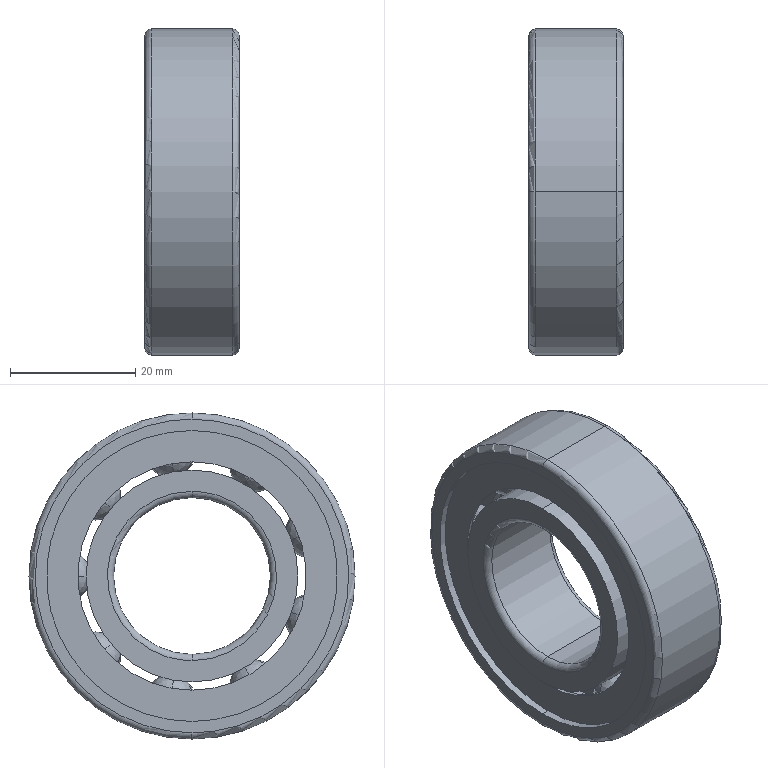Part | NX | features BREP 3 | 3 solids | 127 faces | box 15 x 52 x 52 mm | volume 15248 mm3 | sphere 63 | plane 26 | cylinder 24 | torus 14 | commonest cylinder face diameters 46.4 x8 33.8 x4 36.42 x4 25 x2 37.917 x2 42.283 x2